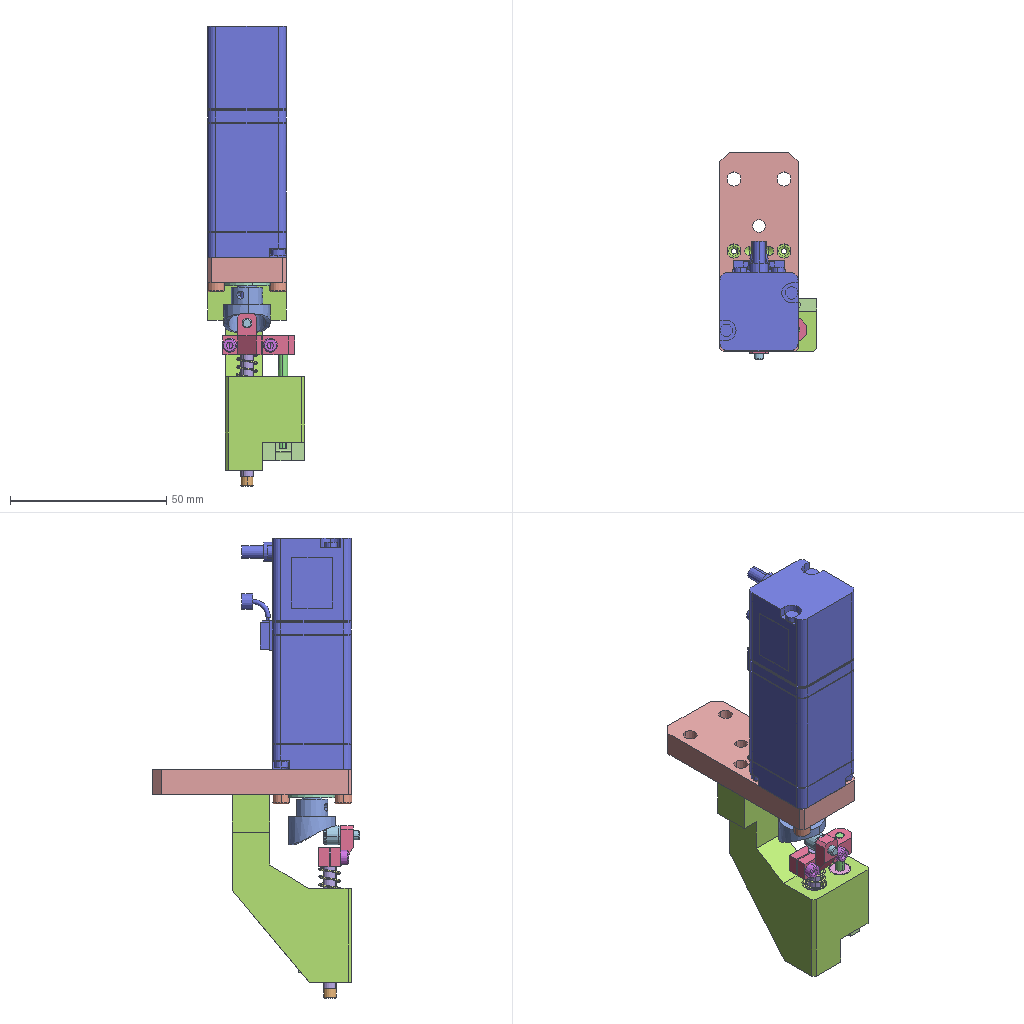Assembly | SolidWorks | 16 different items | 18 placed | box 31 x 66 x 147 mm
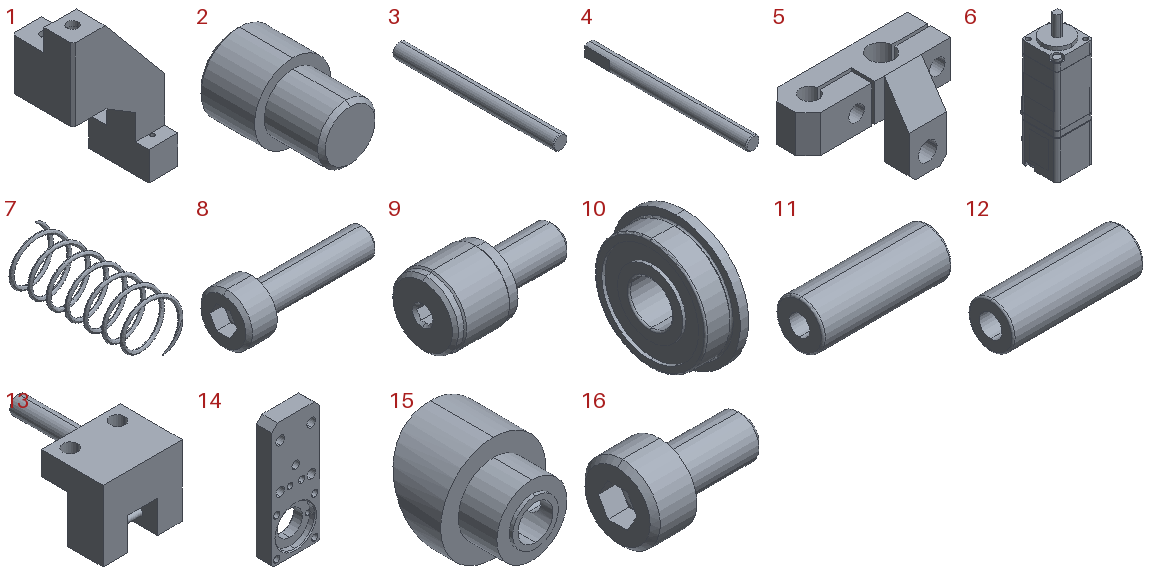Parts list (item | quantity | size | volume | features):
1 | x1 | 38 x 30.9 x 60 mm | 16944 mm3 | features ICE 14, HoleWzd 5, Chamfer 2, Extrusion 1
2 | x1 | 4 x 6 x 4 mm | 58.482 mm3 | features Chamfer 1, Extrusion 1, ICE 1
3 | x1 | 4 x 45 x 4 mm | 544.038 mm3 | features Chamfer 1, Extrusion 1, ICE 1
4 | x1 | 3 x 36 x 3 mm | 245.456 mm3 | features Chamfer 2, Extrusion 1, ICE 1
5 | x1 | 23 x 11 x 13 mm | 943.404 mm3 | features ICE 9, Chamfer 3, Extrusion 1, HoleWzd 1
6 | x1 | 25.2 x 35 x 90 mm | 47544 mm3 | features BaseBody 1, ICE 1
7 | x1 | 7 x 18 x 7 mm | 28.721 mm3 | features Helix 1, ICE 1, RefAxis 1, Sweep 1
8 | x2 | 15 x 5.5 x 5.5 mm | 145.907 mm3 | features ICE 1, RevCut 1, Revolution 1
9 | x1 | 11.5 x 6 x 6 mm | 189.881 mm3 | features ICE 1, RevCut 1, Revolution 1
10 | x1 | 4 x 15 x 15 mm | 450.56 mm3 | features RefAxis 3, 3DProfileFeature 1, Revolution 1
11 | x1 | 19 x 7 x 7 mm | 596.069 mm3 | features Revolution 1
12 | x1 | 23 x 8 x 8 mm | 866.125 mm3 | features RefAxis 3, 3DProfileFeature 1, Revolution 1
13 | x1 | 13.4 x 21 x 12 mm | 1080 mm3 | features ICE 4, Extrusion 1
14 | x1 | 25 x 8 x 63.5 mm | 9911 mm3 | features ICE 6, Chamfer 3, HoleWzd 3, Cut 2, CirPattern 1, Extrusion 1
15 | x1 | 15 x 15 x 15 mm | 872.889 mm3 | features ICE 5, CirPattern 1, Emboss 1, Extrusion 1, HoleWzd 1, RefAxis 1
16 | x2 | 7.5 x 4.5 x 4.5 mm | 58.808 mm3 | features ICE 1, RevCut 1, Revolution 1
Mates (type | each side: item.copy, entity, surface, feature):
Concentric | 3.1 face cylinder Boss-Extrude1 | 5.1 face cylinder Boss-Extrude1
Coincident | 3.1 face plane Boss-Extrude1 | 5.1 face plane Cut-Extrude4
Coincident | 3.1 axis | 7.1 axis
Coincident | 4.1 face plane Boss-Extrude1 | 5.1 face plane Cut-Extrude4
Concentric | 4.1 face cylinder Boss-Extrude1 | 5.1 face cylinder Boss-Extrude1
Concentric | 5.1 face cylinder Cut-Extrude9 | 9.1 face cylinder Revolve1
Coincident | 5.1 face plane Cut-Extrude4 | 9.1 face plane Revolve1
Coincident | 5.1 face plane Boss-Extrude1 | 7.1 face plane Cut-Extrude1
Coincident | 5.1 face plane Cut-Extrude1 | 16.1 face plane Revolve1
Concentric | 5.1 face cylinder Cut-Extrude6 | 16.1 face cylinder Revolve1
Coincident | 5.1 face plane Cut-Extrude1 | 16.2 face plane Revolve1
Concentric | 5.1 face cylinder Cut-Extrude6 | 16.2 face cylinder Revolve1
Coincident | 3.1 face plane Boss-Extrude1 | 2.1 face plane Boss-Extrude2
Concentric | 3.1 face cylinder Boss-Extrude1 | 2.1 face cylinder Boss-Extrude1
Coincident | 14.1 face plane Boss-Extrude1 | 10.1 face plane Revolve1
Concentric | 14.1 face cylinder Cut-Extrude2 | 10.1 face cylinder Revolve1
Coincident | 14.1 face plane Boss-Extrude1 | 8.1 face plane Revolve1
Concentric | 14.1 face cylinder Cut-Extrude5 | 8.1 face cylinder Revolve1
Coincident | 14.1 face plane Boss-Extrude1 | 8.2 face plane Revolve1
Coincident | 14.1 face plane Boss-Extrude1 | 6.1 face plane Imported1 | 2 times
Concentric | 14.1 face cylinder Cut-Extrude2 | 6.1 face cylinder Imported1
Coincident | 15.1 face plane Boss-Extrude3 | 10.1 face plane Revolve1
Concentric | 15.1 face cylinder Cut-Extrude4 | 6.1 face cylinder Imported1
DistanceDim | 5.1 face plane Boss-Extrude1 | 15.1 face plane Boss-Extrude2
Concentric | 1.1 face cylinder Cut-Extrude2 | 12.1 face cylinder Revolve1
Coincident | 1.1 face plane Boss-Extrude2 | 12.1 face plane Revolve1
Coincident | 1.1 face plane Boss-Extrude3 | 11.1 face plane Revolve1
Concentric | 1.1 face cylinder Cut-Extrude2 | 11.1 face cylinder Revolve1
Concentric | 14.1 face cylinder Cut-Extrude7 | 1.1 face cylinder M4 Tapped Hole1 | 2 times
Coincident | 14.1 face plane Boss-Extrude1 | 1.1 face plane Boss-Extrude1
Concentric | 1.1 face cylinder M2 Tapped Hole1 | 13.1 face cylinder Cut-Extrude1 | 2 times
Coincident | 1.1 face plane Cut-Extrude12 | 13.1 face plane Boss-Extrude2
Concentric | 1.1 face cylinder Cut-Extrude2 | 3.1 face cylinder Boss-Extrude1
Concentric | 11.1 face cylinder Revolve1 | 4.1 face cylinder Boss-Extrude1